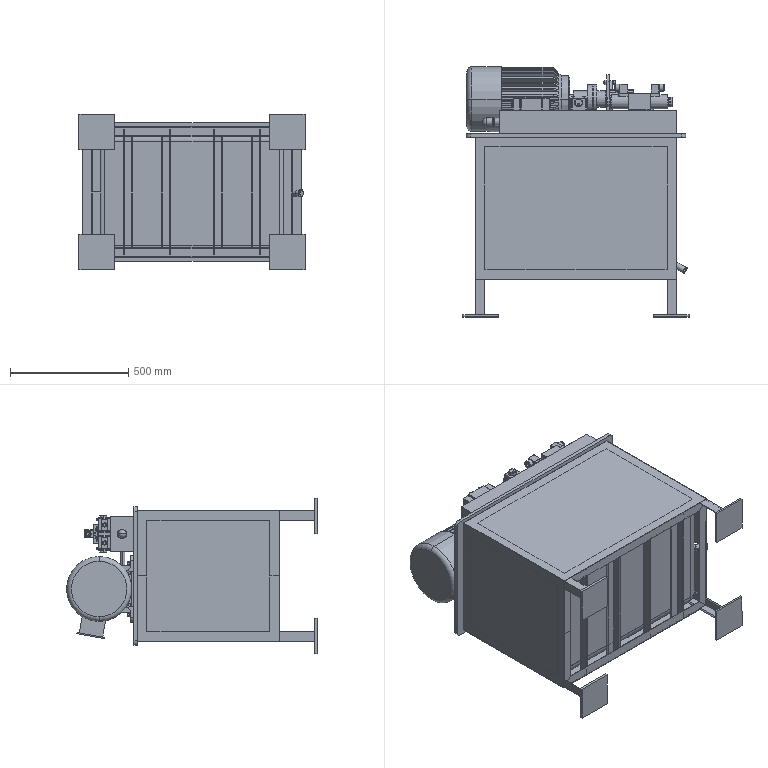Part | SolidWorks | features ReferencePattern 14, CompositeCurve 3, MirrorCompFeat 2 | 99 solids | 2420 faces | box 956 x 1060 x 656 mm | volume 60828027 mm3 | cylinder 1278 | plane 926 | cone 79 | torus 79 | sphere 42 | spline 16 | commonest cylinder face diameters 6 x122 10 x121 2.835 x111 8 x88 4 x69 2 x58